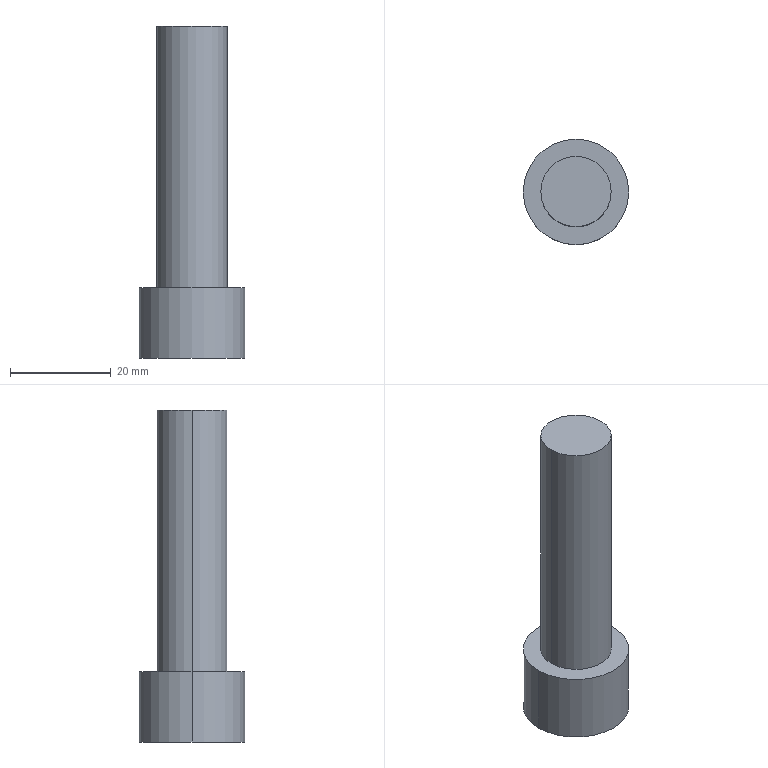Part | Creo | 1 solid | 14 faces | box 21 x 21 x 66 mm | volume 11981 mm3 | plane 10 | cylinder 4 | commonest cylinder face diameters 14 x2 21 x2
STEP:
#1=CARTESIAN_POINT('',(-260.5,-297.,-334.5));
#2=VERTEX_POINT('',#1);
#3=CARTESIAN_POINT('',(-239.5,-297.,-334.5));
#4=VERTEX_POINT('',#3);
#5=CARTESIAN_POINT('',(-250.,-297.,-334.5));
#6=DIRECTION('',(0.,0.,-1.));
#7=DIRECTION('',(-1.,0.,0.));
#8=AXIS2_PLACEMENT_3D('',#5,#6,#7);
#9=CIRCLE('',#8,10.5);
#10=EDGE_CURVE('',#2,#4,#9,.T.);
#11=ORIENTED_EDGE('',*,*,#10,.F.);
#12=CARTESIAN_POINT('',(-250.,-297.,-334.5));
#13=DIRECTION('',(0.,0.,-1.));
#14=DIRECTION('',(1.,0.,0.));
#15=AXIS2_PLACEMENT_3D('',#12,#13,#14);
#16=CIRCLE('',#15,10.5);
#17=EDGE_CURVE('',#4,#2,#16,.T.);
#18=ORIENTED_EDGE('',*,*,#17,.F.);
#19=EDGE_LOOP('',(#11,#18));
#20=FACE_OUTER_BOUND('',#19,.F.);
#21=CARTESIAN_POINT('',(-244.,-293.536,-334.5));
#22=VERTEX_POINT('',#21);
#23=CARTESIAN_POINT('',(-250.,-290.072,-334.5));
#24=VERTEX_POINT('',#23);
#25=CARTESIAN_POINT('',(-244.,-293.536,-334.5));
#26=DIRECTION('',(-0.866,0.5,0.));
#27=VECTOR('',#26,6.928);
#28=LINE('',#25,#27);
#29=EDGE_CURVE('',#22,#24,#28,.T.);
#30=ORIENTED_EDGE('',*,*,#29,.F.);
#31=CARTESIAN_POINT('',(-244.,-300.464,-334.5));
#32=VERTEX_POINT('',#31);
#33=CARTESIAN_POINT('',(-244.,-293.536,-334.5));
#34=DIRECTION('',(0.,-1.,0.));
#35=VECTOR('',#34,6.928);
#36=LINE('',#33,#35);
#37=EDGE_CURVE('',#22,#32,#36,.T.);
#38=ORIENTED_EDGE('',*,*,#37,.T.);
#39=CARTESIAN_POINT('',(-250.,-303.928,-334.5));
#40=VERTEX_POINT('',#39);
#41=CARTESIAN_POINT('',(-250.,-303.928,-334.5));
#42=DIRECTION('',(0.866,0.5,0.));
#43=VECTOR('',#42,6.928);
#44=LINE('',#41,#43);
#45=EDGE_CURVE('',#40,#32,#44,.T.);
#46=ORIENTED_EDGE('',*,*,#45,.F.);
#47=CARTESIAN_POINT('',(-256.,-300.464,-334.5));
#48=VERTEX_POINT('',#47);
#49=CARTESIAN_POINT('',(-256.,-300.464,-334.5));
#50=DIRECTION('',(0.866,-0.5,0.));
#51=VECTOR('',#50,6.928);
#52=LINE('',#49,#51);
#53=EDGE_CURVE('',#48,#40,#52,.T.);
#54=ORIENTED_EDGE('',*,*,#53,.F.);
#55=CARTESIAN_POINT('',(-256.,-293.536,-334.5));
#56=VERTEX_POINT('',#55);
#57=CARTESIAN_POINT('',(-256.,-300.464,-334.5));
#58=DIRECTION('',(0.,1.,0.));
#59=VECTOR('',#58,6.928);
#60=LINE('',#57,#59);
#61=EDGE_CURVE('',#48,#56,#60,.T.);
#62=ORIENTED_EDGE('',*,*,#61,.T.);
#63=CARTESIAN_POINT('',(-250.,-290.072,-334.5));
#64=DIRECTION('',(-0.866,-0.5,0.));
#65=VECTOR('',#64,6.928);
#66=LINE('',#63,#65);
#67=EDGE_CURVE('',#24,#56,#66,.T.);
#68=ORIENTED_EDGE('',*,*,#67,.F.);
#69=EDGE_LOOP('',(#30,#38,#46,#54,#62,#68));
#70=FACE_BOUND('',#69,.F.);
#71=CARTESIAN_POINT('',(-250.,-297.,-334.5));
#72=DIRECTION('',(0.,0.,-1.));
#73=DIRECTION('',(1.,0.,0.));
#74=AXIS2_PLACEMENT_3D('',#71,#72,#73);
#75=PLANE('',#74);
#76=ADVANCED_FACE('',(#20,#70),#75,.T.);
#77=CARTESIAN_POINT('',(-239.5,-297.,-320.5));
#78=VERTEX_POINT('',#77);
#79=CARTESIAN_POINT('',(-260.5,-297.,-320.5));
#80=VERTEX_POINT('',#79);
#81=CARTESIAN_POINT('',(-250.,-297.,-320.5));
#82=DIRECTION('',(0.,0.,1.));
#83=DIRECTION('',(1.,0.,0.));
#84=AXIS2_PLACEMENT_3D('',#81,#82,#83);
#85=CIRCLE('',#84,10.5);
#86=EDGE_CURVE('',#78,#80,#85,.T.);
#87=ORIENTED_EDGE('',*,*,#86,.T.);
#88=CARTESIAN_POINT('',(-260.5,-297.,-334.5));
#89=DIRECTION('',(0.,0.,1.));
#90=VECTOR('',#89,14.);
#91=LINE('',#88,#90);
#92=EDGE_CURVE('',#2,#80,#91,.T.);
#93=ORIENTED_EDGE('',*,*,#92,.F.);
#94=ORIENTED_EDGE('',*,*,#10,.T.);
#95=CARTESIAN_POINT('',(-239.5,-297.,-334.5));
#96=DIRECTION('',(0.,0.,1.));
#97=VECTOR('',#96,14.);
#98=LINE('',#95,#97);
#99=EDGE_CURVE('',#4,#78,#98,.T.);
#100=ORIENTED_EDGE('',*,*,#99,.T.);
#101=EDGE_LOOP('',(#87,#93,#94,#100));
#102=FACE_OUTER_BOUND('',#101,.F.);
#103=CARTESIAN_POINT('',(-250.,-297.,-334.5));
#104=DIRECTION('',(0.,0.,1.));
#105=DIRECTION('',(-1.,0.,0.));
#106=AXIS2_PLACEMENT_3D('',#103,#104,#105);
#107=CYLINDRICAL_SURFACE('',#106,10.5);
#108=ADVANCED_FACE('',(#102),#107,.T.);
#109=ORIENTED_EDGE('',*,*,#86,.F.);
#110=CARTESIAN_POINT('',(-250.,-297.,-320.5));
#111=DIRECTION('',(0.,0.,1.));
#112=DIRECTION('',(-1.,0.,0.));
#113=AXIS2_PLACEMENT_3D('',#110,#111,#112);
#114=CIRCLE('',#113,10.5);
#115=EDGE_CURVE('',#80,#78,#114,.T.);
#116=ORIENTED_EDGE('',*,*,#115,.F.);
#117=EDGE_LOOP('',(#109,#116));
#118=FACE_OUTER_BOUND('',#117,.F.);
#119=CARTESIAN_POINT('',(-257.,-297.,-320.5));
#120=VERTEX_POINT('',#119);
#121=CARTESIAN_POINT('',(-243.,-297.,-320.5));
#122=VERTEX_POINT('',#121);
#123=CARTESIAN_POINT('',(-250.,-297.,-320.5));
#124=DIRECTION('',(0.,0.,-1.));
#125=DIRECTION('',(-1.,0.,0.));
#126=AXIS2_PLACEMENT_3D('',#123,#124,#125);
#127=CIRCLE('',#126,7.);
#128=EDGE_CURVE('',#120,#122,#127,.T.);
#129=ORIENTED_EDGE('',*,*,#128,.F.);
#130=CARTESIAN_POINT('',(-250.,-297.,-320.5));
#131=DIRECTION('',(0.,0.,-1.));
#132=DIRECTION('',(1.,0.,0.));
#133=AXIS2_PLACEMENT_3D('',#130,#131,#132);
#134=CIRCLE('',#133,7.);
#135=EDGE_CURVE('',#122,#120,#134,.T.);
#136=ORIENTED_EDGE('',*,*,#135,.F.);
#137=EDGE_LOOP('',(#129,#136));
#138=FACE_BOUND('',#137,.F.);
#139=CARTESIAN_POINT('',(-250.,-297.,-320.5));
#140=DIRECTION('',(0.,0.,1.));
#141=DIRECTION('',(-1.,0.,0.));
#142=AXIS2_PLACEMENT_3D('',#139,#140,#141);
#143=PLANE('',#142);
#144=ADVANCED_FACE('',(#118,#138),#143,.T.);
#145=ORIENTED_EDGE('',*,*,#128,.T.);
#146=CARTESIAN_POINT('',(-243.,-297.,-268.5));
#147=VERTEX_POINT('',#146);
#148=CARTESIAN_POINT('',(-243.,-297.,-320.5));
#149=DIRECTION('',(0.,0.,1.));
#150=VECTOR('',#149,52.);
#151=LINE('',#148,#150);
#152=EDGE_CURVE('',#122,#147,#151,.T.);
#153=ORIENTED_EDGE('',*,*,#152,.T.);
#154=CARTESIAN_POINT('',(-257.,-297.,-268.5));
#155=VERTEX_POINT('',#154);
#156=CARTESIAN_POINT('',(-250.,-297.,-268.5));
#157=DIRECTION('',(0.,0.,1.));
#158=DIRECTION('',(1.,0.,0.));
#159=AXIS2_PLACEMENT_3D('',#156,#157,#158);
#160=CIRCLE('',#159,7.);
#161=EDGE_CURVE('',#147,#155,#160,.T.);
#162=ORIENTED_EDGE('',*,*,#161,.T.);
#163=CARTESIAN_POINT('',(-257.,-297.,-320.5));
#164=DIRECTION('',(0.,0.,1.));
#165=VECTOR('',#164,52.);
#166=LINE('',#163,#165);
#167=EDGE_CURVE('',#120,#155,#166,.T.);
#168=ORIENTED_EDGE('',*,*,#167,.F.);
#169=EDGE_LOOP('',(#145,#153,#162,#168));
#170=FACE_OUTER_BOUND('',#169,.F.);
#171=CARTESIAN_POINT('',(-250.,-297.,-334.5));
#172=DIRECTION('',(0.,0.,1.));
#173=DIRECTION('',(-1.,0.,0.));
#174=AXIS2_PLACEMENT_3D('',#171,#172,#173);
#175=CYLINDRICAL_SURFACE('',#174,7.);
#176=ADVANCED_FACE('',(#170),#175,.T.);
#177=ORIENTED_EDGE('',*,*,#135,.T.);
#178=ORIENTED_EDGE('',*,*,#167,.T.);
#179=CARTESIAN_POINT('',(-250.,-297.,-268.5));
#180=DIRECTION('',(0.,0.,1.));
#181=DIRECTION('',(-1.,0.,0.));
#182=AXIS2_PLACEMENT_3D('',#179,#180,#181);
#183=CIRCLE('',#182,7.);
#184=EDGE_CURVE('',#155,#147,#183,.T.);
#185=ORIENTED_EDGE('',*,*,#184,.T.);
#186=ORIENTED_EDGE('',*,*,#152,.F.);
#187=EDGE_LOOP('',(#177,#178,#185,#186));
#188=FACE_OUTER_BOUND('',#187,.F.);
#189=CARTESIAN_POINT('',(-250.,-297.,-334.5));
#190=DIRECTION('',(0.,0.,1.));
#191=DIRECTION('',(-1.,0.,0.));
#192=AXIS2_PLACEMENT_3D('',#189,#190,#191);
#193=CYLINDRICAL_SURFACE('',#192,7.);
#194=ADVANCED_FACE('',(#188),#193,.T.);
#195=ORIENTED_EDGE('',*,*,#161,.F.);
#196=ORIENTED_EDGE('',*,*,#184,.F.);
#197=EDGE_LOOP('',(#195,#196));
#198=FACE_OUTER_BOUND('',#197,.F.);
#199=CARTESIAN_POINT('',(-250.,-297.,-268.5));
#200=DIRECTION('',(0.,0.,1.));
#201=DIRECTION('',(-1.,0.,0.));
#202=AXIS2_PLACEMENT_3D('',#199,#200,#201);
#203=PLANE('',#202);
#204=ADVANCED_FACE('',(#198),#203,.T.);
#205=ORIENTED_EDGE('',*,*,#115,.T.);
#206=ORIENTED_EDGE('',*,*,#99,.F.);
#207=ORIENTED_EDGE('',*,*,#17,.T.);
#208=ORIENTED_EDGE('',*,*,#92,.T.);
#209=EDGE_LOOP('',(#205,#206,#207,#208));
#210=FACE_OUTER_BOUND('',#209,.F.);
#211=CARTESIAN_POINT('',(-250.,-297.,-334.5));
#212=DIRECTION('',(0.,0.,1.));
#213=DIRECTION('',(-1.,0.,0.));
#214=AXIS2_PLACEMENT_3D('',#211,#212,#213);
#215=CYLINDRICAL_SURFACE('',#214,10.5);
#216=ADVANCED_FACE('',(#210),#215,.T.);
#217=CARTESIAN_POINT('',(-250.,-290.072,-327.5));
#218=VERTEX_POINT('',#217);
#219=CARTESIAN_POINT('',(-244.,-293.536,-327.5));
#220=VERTEX_POINT('',#219);
#221=CARTESIAN_POINT('',(-250.,-290.072,-327.5));
#222=DIRECTION('',(0.866,-0.5,0.));
#223=VECTOR('',#222,6.928);
#224=LINE('',#221,#223);
#225=EDGE_CURVE('',#218,#220,#224,.T.);
#226=ORIENTED_EDGE('',*,*,#225,.T.);
#227=CARTESIAN_POINT('',(-244.,-293.536,-327.5));
#228=DIRECTION('',(0.,0.,-1.));
#229=VECTOR('',#228,7.);
#230=LINE('',#227,#229);
#231=EDGE_CURVE('',#220,#22,#230,.T.);
#232=ORIENTED_EDGE('',*,*,#231,.T.);
#233=ORIENTED_EDGE('',*,*,#29,.T.);
#234=CARTESIAN_POINT('',(-250.,-290.072,-327.5));
#235=DIRECTION('',(0.,0.,-1.));
#236=VECTOR('',#235,7.);
#237=LINE('',#234,#236);
#238=EDGE_CURVE('',#218,#24,#237,.T.);
#239=ORIENTED_EDGE('',*,*,#238,.F.);
#240=EDGE_LOOP('',(#226,#232,#233,#239));
#241=FACE_OUTER_BOUND('',#240,.F.);
#242=CARTESIAN_POINT('',(-247.,-291.804,-331.));
#243=DIRECTION('',(0.5,0.866,0.));
#244=DIRECTION('',(-0.866,0.5,0.));
#245=AXIS2_PLACEMENT_3D('',#242,#243,#244);
#246=PLANE('',#245);
#247=ADVANCED_FACE('',(#241),#246,.F.);
#248=CARTESIAN_POINT('',(-244.,-300.464,-327.5));
#249=VERTEX_POINT('',#248);
#250=CARTESIAN_POINT('',(-244.,-293.536,-327.5));
#251=DIRECTION('',(0.,-1.,0.));
#252=VECTOR('',#251,6.928);
#253=LINE('',#250,#252);
#254=EDGE_CURVE('',#220,#249,#253,.T.);
#255=ORIENTED_EDGE('',*,*,#254,.F.);
#256=ORIENTED_EDGE('',*,*,#225,.F.);
#257=CARTESIAN_POINT('',(-256.,-293.536,-327.5));
#258=VERTEX_POINT('',#257);
#259=CARTESIAN_POINT('',(-256.,-293.536,-327.5));
#260=DIRECTION('',(0.866,0.5,0.));
#261=VECTOR('',#260,6.928);
#262=LINE('',#259,#261);
#263=EDGE_CURVE('',#258,#218,#262,.T.);
#264=ORIENTED_EDGE('',*,*,#263,.F.);
#265=CARTESIAN_POINT('',(-256.,-300.464,-327.5));
#266=VERTEX_POINT('',#265);
#267=CARTESIAN_POINT('',(-256.,-300.464,-327.5));
#268=DIRECTION('',(0.,1.,0.));
#269=VECTOR('',#268,6.928);
#270=LINE('',#267,#269);
#271=EDGE_CURVE('',#266,#258,#270,.T.);
#272=ORIENTED_EDGE('',*,*,#271,.F.);
#273=CARTESIAN_POINT('',(-250.,-303.928,-327.5));
#274=VERTEX_POINT('',#273);
#275=CARTESIAN_POINT('',(-250.,-303.928,-327.5));
#276=DIRECTION('',(-0.866,0.5,0.));
#277=VECTOR('',#276,6.928);
#278=LINE('',#275,#277);
#279=EDGE_CURVE('',#274,#266,#278,.T.);
#280=ORIENTED_EDGE('',*,*,#279,.F.);
#281=CARTESIAN_POINT('',(-244.,-300.464,-327.5));
#282=DIRECTION('',(-0.866,-0.5,0.));
#283=VECTOR('',#282,6.928);
#284=LINE('',#281,#283);
#285=EDGE_CURVE('',#249,#274,#284,.T.);
#286=ORIENTED_EDGE('',*,*,#285,.F.);
#287=EDGE_LOOP('',(#255,#256,#264,#272,#280,#286));
#288=FACE_OUTER_BOUND('',#287,.F.);
#289=CARTESIAN_POINT('',(-250.,-297.,-327.5));
#290=DIRECTION('',(0.,0.,1.));
#291=DIRECTION('',(-1.,0.,0.));
#292=AXIS2_PLACEMENT_3D('',#289,#290,#291);
#293=PLANE('',#292);
#294=ADVANCED_FACE('',(#288),#293,.F.);
#295=ORIENTED_EDGE('',*,*,#254,.T.);
#296=CARTESIAN_POINT('',(-244.,-300.464,-327.5));
#297=DIRECTION('',(0.,0.,-1.));
#298=VECTOR('',#297,7.);
#299=LINE('',#296,#298);
#300=EDGE_CURVE('',#249,#32,#299,.T.);
#301=ORIENTED_EDGE('',*,*,#300,.T.);
#302=ORIENTED_EDGE('',*,*,#37,.F.);
#303=ORIENTED_EDGE('',*,*,#231,.F.);
#304=EDGE_LOOP('',(#295,#301,#302,#303));
#305=FACE_OUTER_BOUND('',#304,.F.);
#306=CARTESIAN_POINT('',(-244.,-297.,-331.));
#307=DIRECTION('',(1.,0.,0.));
#308=DIRECTION('',(0.,0.,1.));
#309=AXIS2_PLACEMENT_3D('',#306,#307,#308);
#310=PLANE('',#309);
#311=ADVANCED_FACE('',(#305),#310,.F.);
#312=ORIENTED_EDGE('',*,*,#285,.T.);
#313=CARTESIAN_POINT('',(-250.,-303.928,-327.5));
#314=DIRECTION('',(0.,0.,-1.));
#315=VECTOR('',#314,7.);
#316=LINE('',#313,#315);
#317=EDGE_CURVE('',#274,#40,#316,.T.);
#318=ORIENTED_EDGE('',*,*,#317,.T.);
#319=ORIENTED_EDGE('',*,*,#45,.T.);
#320=ORIENTED_EDGE('',*,*,#300,.F.);
#321=EDGE_LOOP('',(#312,#318,#319,#320));
#322=FACE_OUTER_BOUND('',#321,.F.);
#323=CARTESIAN_POINT('',(-247.,-302.196,-331.));
#324=DIRECTION('',(0.5,-0.866,0.));
#325=DIRECTION('',(0.866,0.5,0.));
#326=AXIS2_PLACEMENT_3D('',#323,#324,#325);
#327=PLANE('',#326);
#328=ADVANCED_FACE('',(#322),#327,.F.);
#329=ORIENTED_EDGE('',*,*,#279,.T.);
#330=CARTESIAN_POINT('',(-256.,-300.464,-327.5));
#331=DIRECTION('',(0.,0.,-1.));
#332=VECTOR('',#331,7.);
#333=LINE('',#330,#332);
#334=EDGE_CURVE('',#266,#48,#333,.T.);
#335=ORIENTED_EDGE('',*,*,#334,.T.);
#336=ORIENTED_EDGE('',*,*,#53,.T.);
#337=ORIENTED_EDGE('',*,*,#317,.F.);
#338=EDGE_LOOP('',(#329,#335,#336,#337));
#339=FACE_OUTER_BOUND('',#338,.F.);
#340=CARTESIAN_POINT('',(-253.,-302.196,-331.));
#341=DIRECTION('',(-0.5,-0.866,0.));
#342=DIRECTION('',(0.866,-0.5,0.));
#343=AXIS2_PLACEMENT_3D('',#340,#341,#342);
#344=PLANE('',#343);
#345=ADVANCED_FACE('',(#339),#344,.F.);
#346=ORIENTED_EDGE('',*,*,#271,.T.);
#347=CARTESIAN_POINT('',(-256.,-293.536,-327.5));
#348=DIRECTION('',(0.,0.,-1.));
#349=VECTOR('',#348,7.);
#350=LINE('',#347,#349);
#351=EDGE_CURVE('',#258,#56,#350,.T.);
#352=ORIENTED_EDGE('',*,*,#351,.T.);
#353=ORIENTED_EDGE('',*,*,#61,.F.);
#354=ORIENTED_EDGE('',*,*,#334,.F.);
#355=EDGE_LOOP('',(#346,#352,#353,#354));
#356=FACE_OUTER_BOUND('',#355,.F.);
#357=CARTESIAN_POINT('',(-256.,-297.,-331.));
#358=DIRECTION('',(-1.,0.,0.));
#359=DIRECTION('',(0.,0.,-1.));
#360=AXIS2_PLACEMENT_3D('',#357,#358,#359);
#361=PLANE('',#360);
#362=ADVANCED_FACE('',(#356),#361,.F.);
#363=ORIENTED_EDGE('',*,*,#263,.T.);
#364=ORIENTED_EDGE('',*,*,#238,.T.);
#365=ORIENTED_EDGE('',*,*,#67,.T.);
#366=ORIENTED_EDGE('',*,*,#351,.F.);
#367=EDGE_LOOP('',(#363,#364,#365,#366));
#368=FACE_OUTER_BOUND('',#367,.F.);
#369=CARTESIAN_POINT('',(-253.,-291.804,-331.));
#370=DIRECTION('',(-0.5,0.866,0.));
#371=DIRECTION('',(-0.866,-0.5,0.));
#372=AXIS2_PLACEMENT_3D('',#369,#370,#371);
#373=PLANE('',#372);
#374=ADVANCED_FACE('',(#368),#373,.F.);
#375=CLOSED_SHELL('',(#76,#108,#144,#176,#194,#204,#216,#247,#294,#311,#328,#345,#362,#374));
#376=MANIFOLD_SOLID_BREP('',#375);
#377=(LENGTH_UNIT()NAMED_UNIT(*)SI_UNIT(.MILLI.,.METRE.));
#378=UNCERTAINTY_MEASURE_WITH_UNIT(LENGTH_MEASURE(0.007238),#377,'','');
#379=(NAMED_UNIT(*)PLANE_ANGLE_UNIT()SI_UNIT($,.RADIAN.));
#380=PLANE_ANGLE_MEASURE_WITH_UNIT(PLANE_ANGLE_MEASURE(0.01745),#379);
#381=(CONVERSION_BASED_UNIT('DEGREE',#380)NAMED_UNIT(*)PLANE_ANGLE_UNIT());
#382=(NAMED_UNIT(*)SI_UNIT($,.STERADIAN.)SOLID_ANGLE_UNIT());
#383=(GEOMETRIC_REPRESENTATION_CONTEXT(3)GLOBAL_UNCERTAINTY_ASSIGNED_CONTEXT((#378))GLOBAL_UNIT_ASSIGNED_CONTEXT((#377,#381,#382))REPRESENTATION_CONTEXT('',''));
#384=ADVANCED_BREP_SHAPE_REPRESENTATION('',(#376),#383);